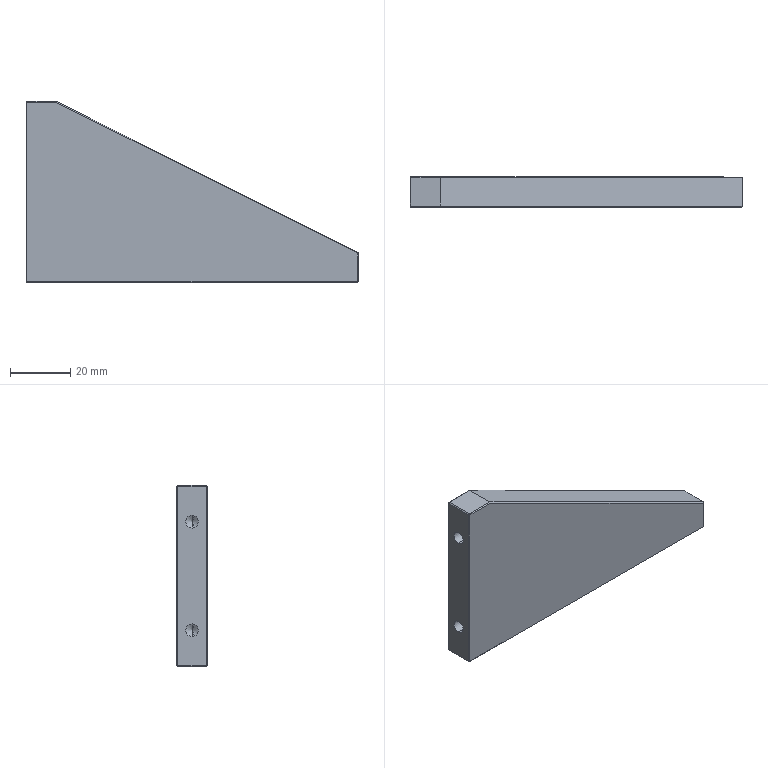Part | STEP file | ND25021-01-JDKM-44-TL | 1 solid | 42 faces | box 110 x 10 x 60 mm | volume 40261 mm3 | plane 26 | cylinder 8 | cone 8 | commonest cylinder face diameters 4.2 x8